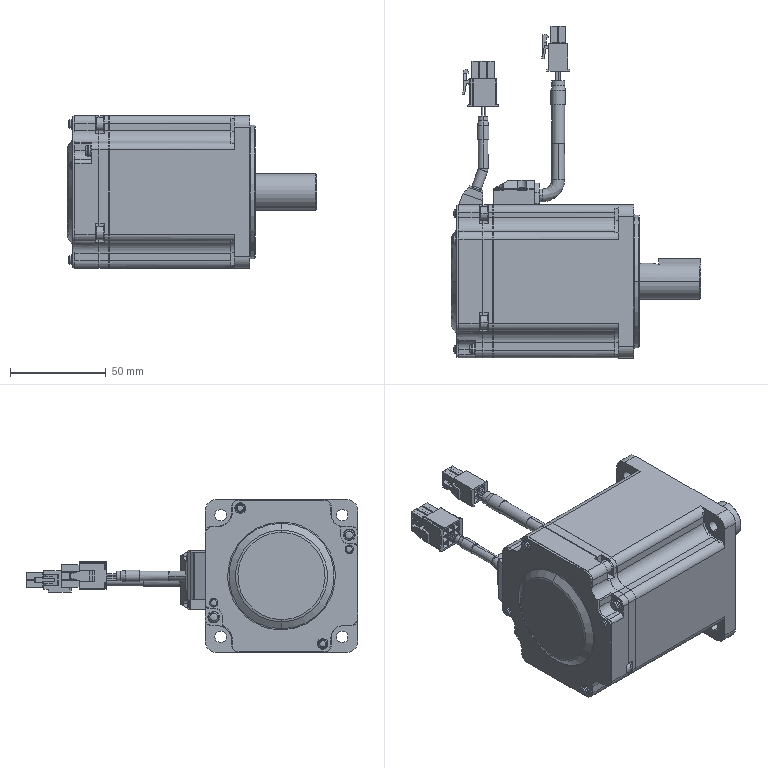Part | SolidWorks | 7 solids | 912 faces | box 130.4 x 173.65 x 80 mm | volume 566555 mm3 | plane 513 | cylinder 294 | cone 59 | spline 46 | commonest cylinder face diameters 8 x32 1 x30 2.6 x26 6 x15 7.84 x12 0.2 x10